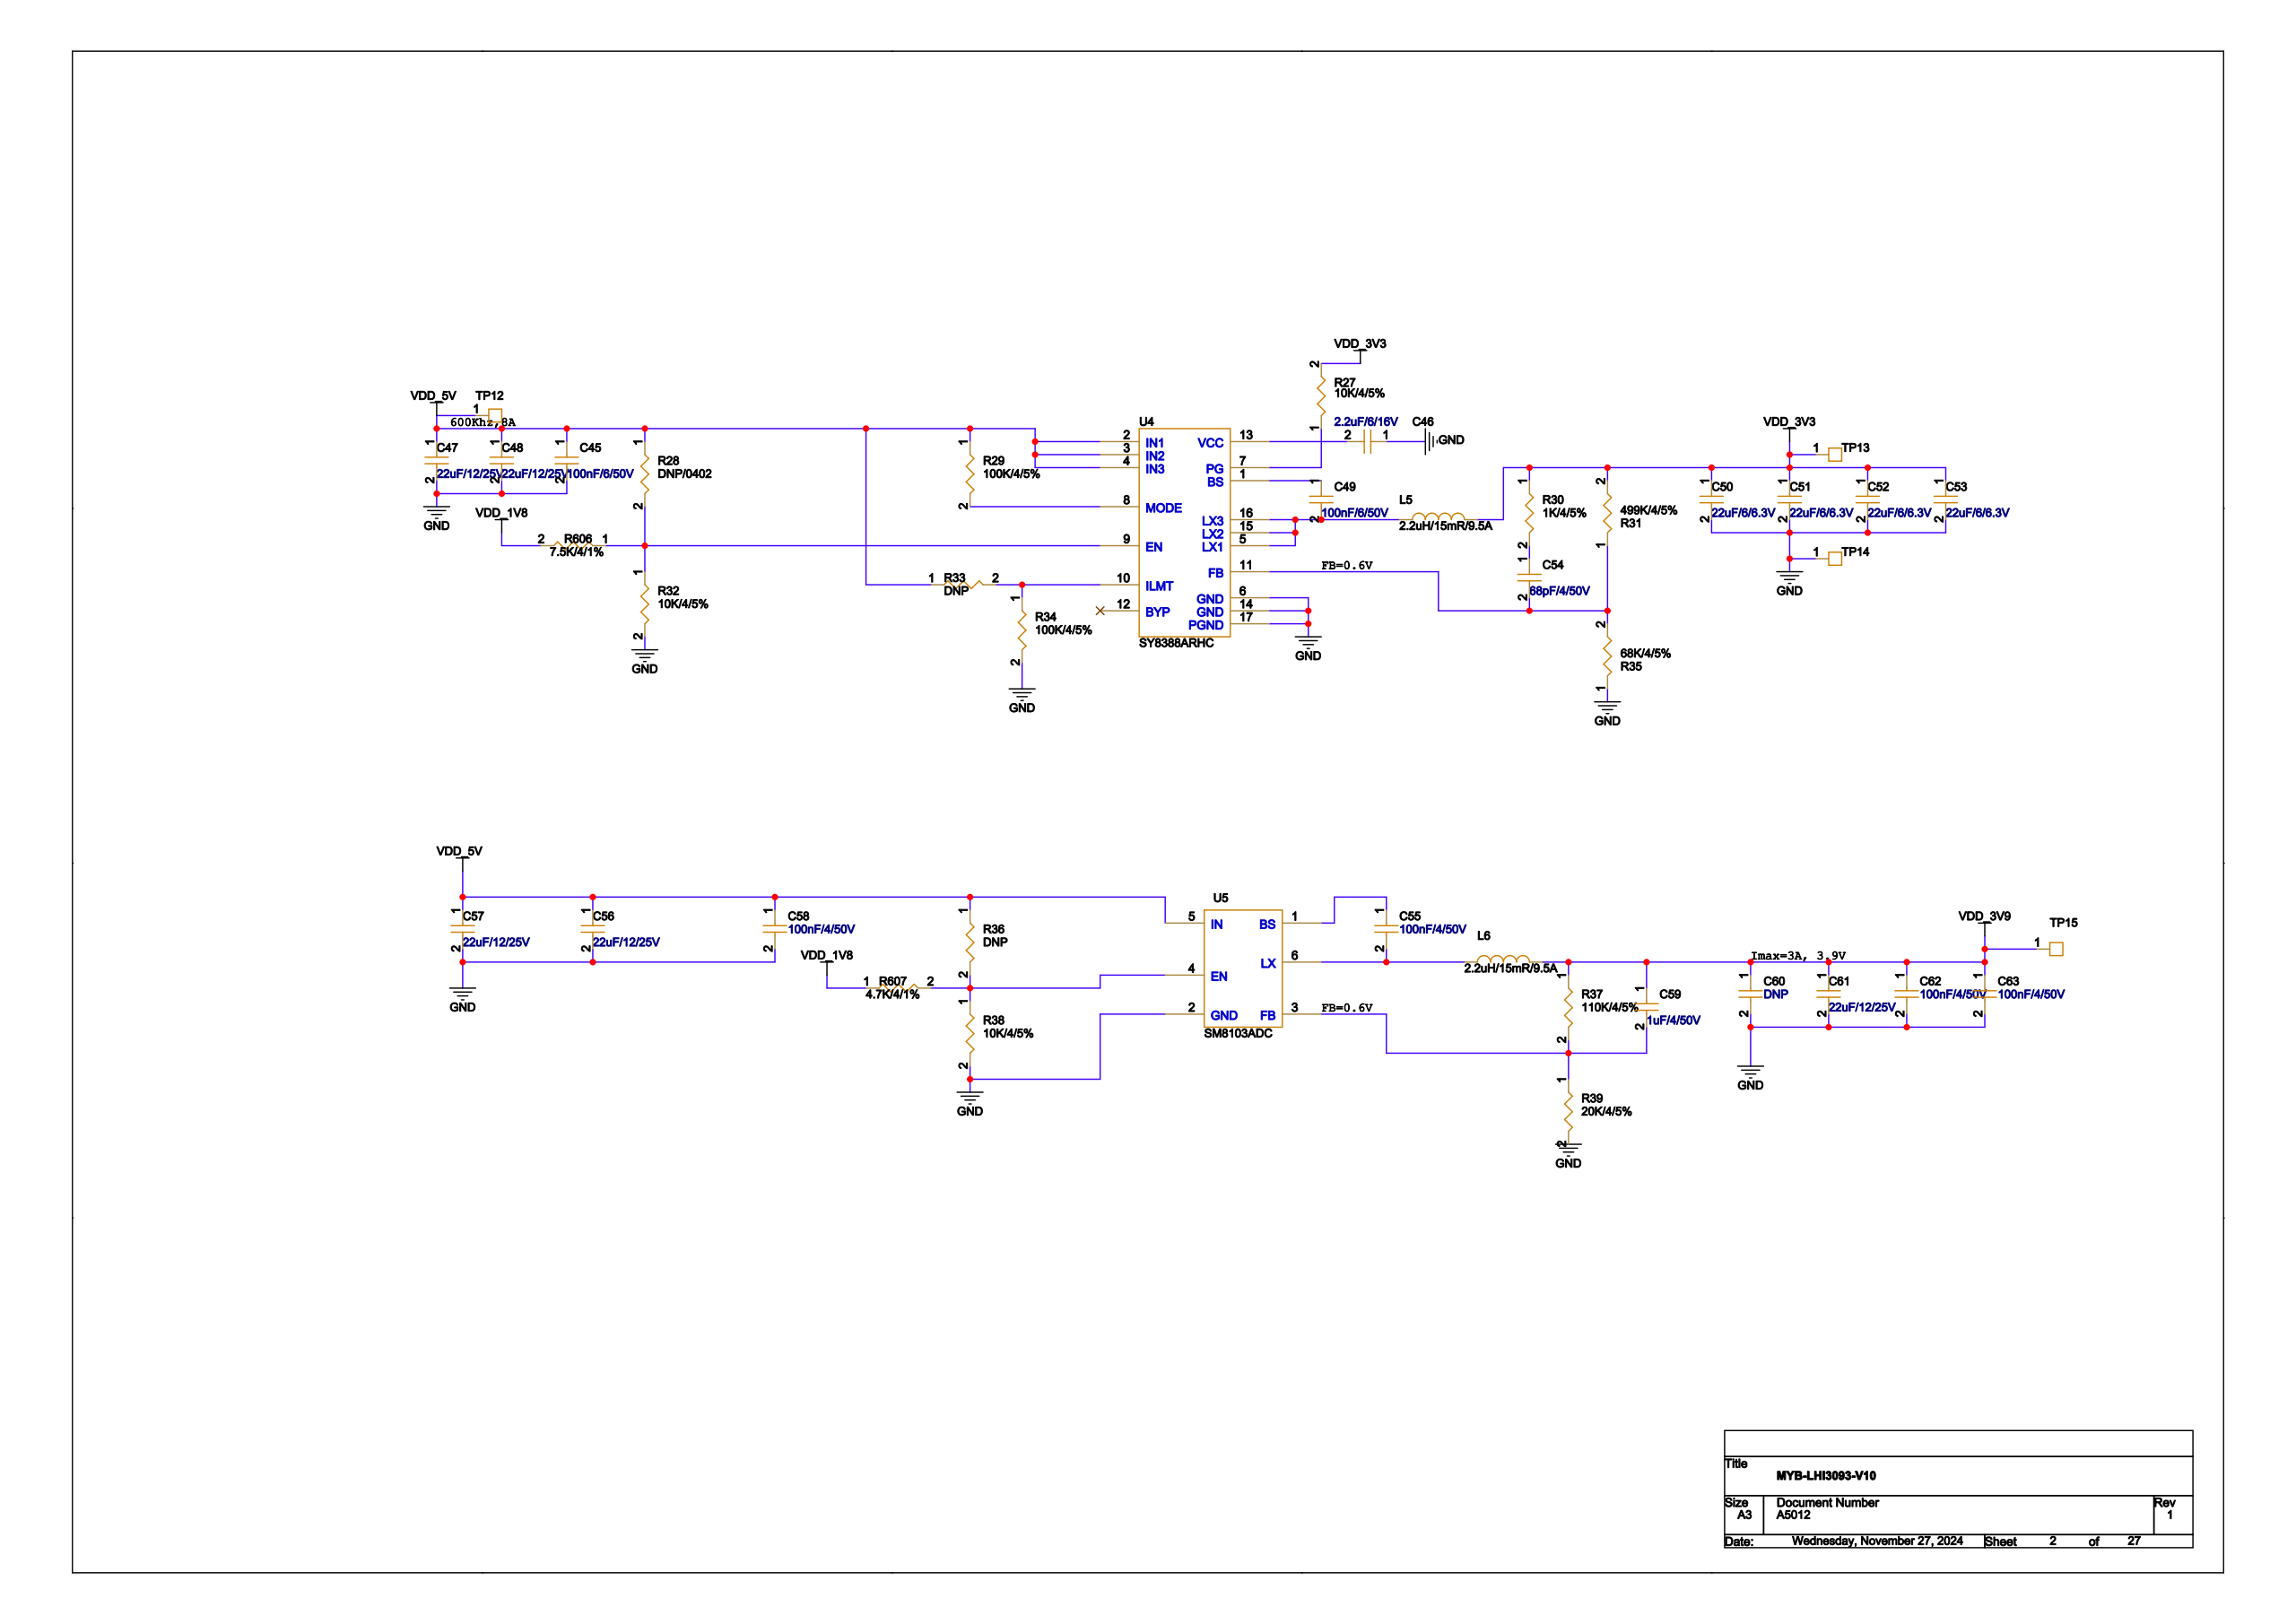Circuit board | Cadence Allegro | 1159 parts | 708 nets | one sheet of the schematic
Parts on this sheet (reference | value | footprint):
C45 | 100nF/6/50V | C0603
C46 | 2.2uF/6/16V | C0603
C47 | 22uF/12/25V | C1206
C48 | 22uF/12/25V | C1206
C49 | 100nF/6/50V | C0603
C50 | 22uF/6/6.3V | C0603
C51 | 22uF/6/6.3V | C0603
C52 | 22uF/6/6.3V | C0603
C53 | 22uF/6/6.3V | C0603
C54 | 68pF/4/50V | C0402
C55 | 100nF/4/50V | C0402
C56 | 22uF/12/25V | C1206
C57 | 22uF/12/25V | C1206
C58 | 100nF/4/50V | C0402
C59 | 1uF/4/50V | C0402
C60 | DNP | C1206
C61 | 22uF/12/25V | C1206
C62 | 100nF/4/50V | C0402
C63 | 100nF/4/50V | C0402
L5 | 2.2uH/15mR/9.5A | L7X6_6
L6 | 2.2uH/15mR/9.5A | L5_2X5_5
R27 | 10K/4/5% | R0402
R28 | DNP/0402 | R0402
R29 | 100K/4/5% | R0402
R30 | 1K/4/5% | R0402
R31 | 499K/4/5% | R0402
R32 | 10K/4/5% | R0402
R33 | DNP | R0402
R34 | 100K/4/5% | R0402
R35 | 68K/4/5% | R0402
R36 | DNP | R0402
R37 | 110K/4/5% | R0402
R38 | 10K/4/5% | R0402
R39 | 20K/4/5% | R0402
R606 | 7.5K/4/1% | R0402
R607 | 4.7K/4/1% | R0402
TP12 | T POINT S | TPAD_020
TP13 | T POINT S | TPAD_020
TP14 | T POINT S | TPAD_020
TP15 | T POINT S | HOLE-TP0_9S16
U4 | SY8388ARHC | QFN16_0_45
U5 | SM8103ADC | SOT23-6
Nets of these parts (net: part-pin ...):
GND: C45-2 C46-1 C47-2 C48-2 C50-2 C51-2 C52-2 C53-2 C56-2 C57-2 C58-2 C60-2 C61-2 C62-2 C63-2 R32-2 R34-2 R35-1 R38-2 R39-2 TP14-1 U4-6 U4-14 U4-17 U5-2
VDD_5V: C45-1 C47-1 C48-1 C56-1 C57-1 C58-1 R28-1 R29-1 R33-1 R36-1 TP12-1 U4-2 U4-3 U4-4 U5-5
VDD_3V9: C59-1 C60-1 C61-1 C62-1 C63-1 L6-2 R37-1 TP15-1
VDD_3V3: C50-1 C51-1 C52-1 C53-1 L5-2 R27-2 R30-1 R31-2 TP13-1
VDD_1V8: R606-2 R607-1
N14923921: C55-1 U5-1
N14923959: C55-2 L6-1 U5-6
N14914520: C46-2 U4-13
N14914580: C49-1 U4-1
N14914584: C49-2 L5-1 U4-5 U4-15 U4-16
N14914648: C54-1 R30-2
N14914632: C54-2 R31-1 R35-2 U4-11
N14924039: C59-2 R37-2 R39-1 U5-3
N14914348: R29-2 U4-8
N14914404: R33-2 R34-1 U4-10
N14914484: R27-1 U4-7
N14914296: R28-2 R32-1 R606-1 U4-9
N14923873: R36-2 R38-1 R607-2 U5-4